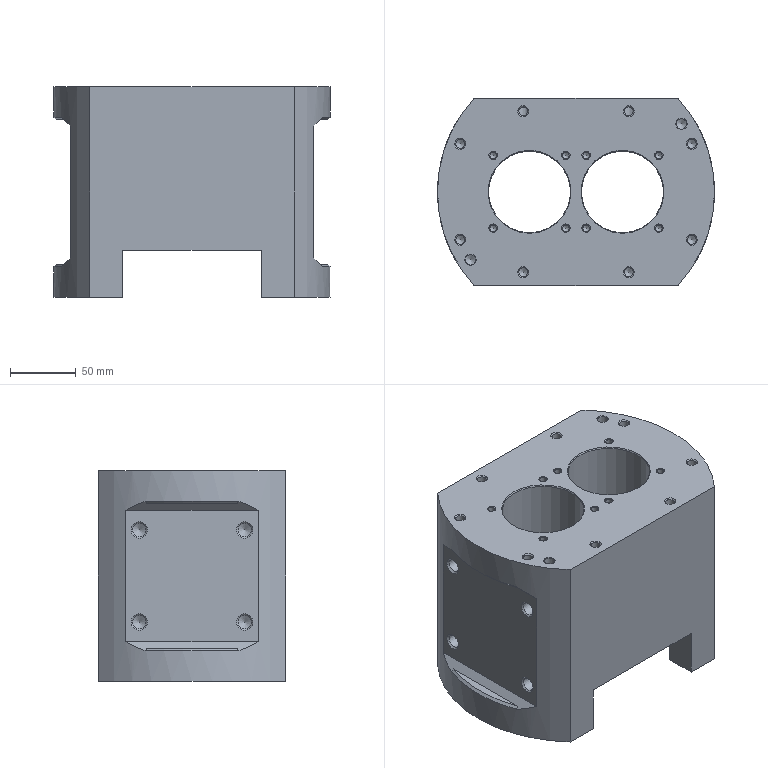NC program | NX | posted with a generic post | part box 210 x 142 x 160 mm
Lines 2091 to 2948 of 4789:
(ZLEVEL_PROFILE , TOOL : D6R0.5)
N4168 T05 M6
N4170 G54
N4172 G17 G0 G90 X-53.624 Y12.863 B0. C0. S6500 M3
N4174 G43 Z30. H5
N4176 Z2.929
N4178 G94 G1 Z-0.071 F1000.
N4180 X-54.42 Y12.281
N4182 G3 X-54.662 Y11.732 R0.6
N4184 G2 X-54.662 Y-11.732 R108.942 F2500.
N4186 G1 X-54.661 Y-11.887 Z-0.088
N4188 Y-12.042 Z-0.106
N4190 X-54.662 Y-12.197 Z-0.124
N4192 X-54.665 Y-12.352 Z-0.141
N4194 G3 X-54.665 Y12.356 R108.252
N4196 G1 X-54.663 Y12.506 Z-0.159
N4198 Y12.657 Z-0.177
N4200 X-54.664 Y12.807 Z-0.194
N4202 X-54.667 Y12.957 Z-0.212
N4204 G2 X-54.667 Y-12.956 R107.872
N4206 G1 X-54.664 Y-13.103 Z-0.23
N4208 X-54.665 Y-13.25 Z-0.247
N4210 Y-13.397 Z-0.265
N4212 X-54.667 Y-13.544 Z-0.283
N4214 G3 X-54.667 Y13.543 R108.056
N4216 G1 X-54.666 Y13.687 Z-0.301
N4218 X-54.667 Y13.832 Z-0.318
N4220 Y13.976 Z-0.336
N4222 X-54.669 Y14.12 Z-0.354
N4224 G2 X-54.668 Y-14.125 R108.36
N4226 G1 X-54.666 Y-14.262 Z-0.371
N4228 Y-14.4 Z-0.389
N4230 X-54.667 Y-14.537 Z-0.407
N4232 X-54.671 Y-14.674 Z-0.424
N4234 G3 X-54.671 Y14.674 R108.329
N4236 G1 X-54.667 Y14.844 Z-0.448
N4238 X-54.668 Y15.014 Z-0.471
N4240 X-54.671 Y15.183 Z-0.495
N4242 G2 X-54.671 Y-15.179 R107.83
N4244 G1 Y-15.344 Z-0.519
N4246 Y-15.508 Z-0.542
N4248 X-54.674 Y-15.672 Z-0.566
N4250 G3 X-54.674 Y15.674 R107.881
N4252 G1 X-54.672 Y15.836 Z-0.589
N4254 Y15.998 Z-0.613
N4256 X-54.675 Y16.159 Z-0.636
N4258 G2 X-54.675 Y-16.159 R107.965
N4260 G1 X-54.673 Y-16.318 Z-0.66
N4262 X-54.674 Y-16.477 Z-0.684
N4264 X-54.675 Y-16.635 Z-0.707
N4266 G3 X-54.675 Y16.633 R108.191
N4268 G1 Y16.79 Z-0.731
N4270 Y16.947 Z-0.754
N4272 X-54.679 Y17.103 Z-0.778
N4274 G2 X-54.678 Y-17.106 R108.255
N4276 G1 X-54.675 Y-17.257 Z-0.801
N4278 X-54.676 Y-17.407 Z-0.825
N4280 X-54.679 Y-17.557 Z-0.849
N4282 G3 X-54.679 Y17.556 R108.476
N4284 G1 X-54.677 Y17.701 Z-0.872
N4286 Y17.846 Z-0.896
N4288 X-54.679 Y17.991 Z-0.919
N4290 G2 X-54.679 Y-17.987 R108.599
N4292 G1 Y-18.125 Z-0.943
N4294 X-54.68 Y-18.263 Z-0.966
N4296 X-54.682 Y-18.401 Z-0.99
N4298 G3 X-54.682 Y18.403 R108.317
N4300 G1 X-54.681 Y18.541 Z-1.014
N4302 Y18.679 Z-1.037
N4304 X-54.685 Y18.816 Z-1.061
N4306 G2 X-54.685 Y-18.815 R108.248
N4308 G1 X-54.682 Y-18.951 Z-1.084
N4310 X-54.683 Y-19.086 Z-1.108
N4312 X-54.686 Y-19.221 Z-1.131
N4314 G3 X-54.686 Y19.221 R108.279
N4316 G1 X-54.684 Y19.354 Z-1.155
N4318 X-54.685 Y19.488 Z-1.179
N4320 X-54.687 Y19.62 Z-1.202
N4322 G2 X-54.687 Y-19.622 R108.38
N4324 G1 X-54.685 Y-19.756 Z-1.226
N4326 Y-19.89 Z-1.249
N4328 X-54.687 Y-20.023 Z-1.273
N4330 G3 X-54.687 Y20.019 R108.652
N4332 G1 X-54.686 Y20.146 Z-1.296
N4334 X-54.687 Y20.274 Z-1.32
N4336 X-54.688 Y20.401 Z-1.344
N4338 G2 X-54.688 Y-20.401 R108.747
N4340 G1 Y-20.526 Z-1.367
N4342 X-54.689 Y-20.651 Z-1.391
N4344 X-54.69 Y-20.775 Z-1.414
N4346 G3 X-54.689 Y20.778 R108.773
N4348 G1 Y20.897 Z-1.438
N4350 X-54.69 Y21.015 Z-1.461
N4352 X-54.691 Y21.134 Z-1.485
N4354 G2 X-54.691 Y-21.132 R108.6
N4356 G1 Y-21.251 Z-1.508
N4358 Y-21.37 Z-1.532
N4360 X-54.693 Y-21.488 Z-1.556
N4362 G3 X-54.693 Y21.49 R108.595
N4364 G1 X-54.692 Y21.608 Z-1.579
N4366 X-54.693 Y21.726 Z-1.603
N4368 X-54.694 Y21.843 Z-1.626
N4370 G2 X-54.694 Y-21.843 R108.602
N4372 G1 Y-22.016 Z-1.662
N4374 X-54.695 Y-22.189 Z-1.697
N4376 G3 X-54.695 Y22.188 R108.586
N4378 G1 Y22.359 Z-1.732
N4380 X-54.696 Y22.53 Z-1.768
N4382 G2 X-52.49 Y-5.881 R108.942
N4384 X-54.696 Y-22.532 R111.727
N4386 G1 X-54.695 Y-22.703 Z-1.803
N4388 X-54.696 Y-22.874 Z-1.838
N4390 G3 X-52.291 Y-2.768 R111.408
N4392 X-54.697 Y22.872 R109.772
N4394 G1 X-54.696 Y23.036 Z-1.874
N4396 X-54.697 Y23.199 Z-1.909
N4398 G2 X-52.184 Y0. R110.754
N4400 X-54.697 Y-23.2 R110.742
N4402 G1 Y-23.361 Z-1.945
N4404 Y-23.523 Z-1.98
N4406 G3 X-52.15 Y-2.768 R111.476
N4408 X-54.697 Y23.525 R110.138
N4410 G1 X-54.696 Y23.683 Z-2.015
N4412 X-54.698 Y23.84 Z-2.051
N4414 G2 X-52.147 Y4.497 R110.747
N4416 X-52.188 Y-5.535 R122.613
N4418 X-54.699 Y-23.836 R112.131
N4420 G1 X-54.698 Y-23.991 Z-2.086
N4422 X-54.7 Y-24.145 Z-2.121
N4424 G3 X-52.12 Y-5.535 R111.408
N4426 X-52.12 Y5.535 R174.408
N4428 X-54.7 Y24.147 R111.521
N4430 G1 X-54.699 Y24.301 Z-2.157
N4432 X-54.702 Y24.454 Z-2.192
N4434 G2 X-52.227 Y8.302 R112.523
N4436 X-52.055 Y4.784 R58.069
N4438 X-52.07 Y-5.535 R256.368
N4440 X-53.483 Y-18.335 R102.106
N4442 X-54.702 Y-24.453 R104.408
N4444 G1 X-54.7 Y-24.608 Z-2.228
N4446 X-54.703 Y-24.761 Z-2.263
N4448 G3 X-52.157 Y-8.302 R112.193
N4450 X-52.023 Y-4.71 R68.447
N4452 X-52.023 Y4.71 R497.71
N4454 X-52.157 Y8.302 R68.447
N4456 X-54.703 Y24.761 R112.204
N4458 G1 X-54.701 Y24.916 Z-2.299
N4460 X-54.704 Y25.069 Z-2.334
N4462 G2 X-52.097 Y8.302 R109.925
N4464 X-52. Y3.907 R99.302
N4466 G1 Y-3.907
N4468 G2 X-52.097 Y-8.302 R99.301
N4470 X-54.704 Y-25.069 R109.989
N4472 G1 X-54.702 Y-25.224 Z-2.37
N4474 X-54.705 Y-25.378 Z-2.405
N4476 G3 X-53.78 Y-21.102 R106.125
N4478 X-52.092 Y-8.994 R103.684
N4480 X-52. Y-5.563 R64.244
N4482 G1 Y4.497
N4484 G3 X-52.056 Y8.302 R101.819
N4486 X-52.268 Y11.07 R47.31
N4488 X-54.705 Y25.376 R113.821
N4490 G1 X-54.703 Y25.529 Z-2.441
N4492 X-54.706 Y25.681 Z-2.476
N4494 G2 X-52.203 Y11.125 R114.465
N4496 X-52.021 Y8.052 R33.208
N4498 G1 X-52.002 Y6.573
N4500 X-52.001 Y6.227
N4502 X-52. Y6.031
N4504 Y-6.04
N4506 X-52.002 Y-6.573
N4508 X-52.021 Y-8.036
N4510 G2 X-52.207 Y-11.158 R33.543
N4512 X-54.705 Y-25.683 R115.071
N4514 G1 X-54.704 Y-25.831 Z-2.512
N4516 X-54.706 Y-25.978 Z-2.547
N4518 G3 X-52.164 Y-11.416 R115.432
N4520 X-52.002 Y-7.611 R42.565
N4522 G1 X-52.001 Y-7.265
N4524 X-52. Y-7.142
N4526 Y7.145
N4528 X-52.001 Y7.265
N4530 X-52.002 Y7.611
N4532 G3 X-52.164 Y11.416 R42.565
N4534 X-54.706 Y25.977 R114.96
N4536 G1 Y26.124 Z-2.583
N4538 X-54.707 Y26.27 Z-2.619
N4540 G2 X-52.137 Y11.762 R113.314
N4542 X-52.003 Y8.648 R35.799
N4544 G1 X-52.001 Y8.302
N4546 X-52. Y8.103
N4548 Y-8.105
N4550 X-52.001 Y-8.302
N4552 X-52.003 Y-8.648
N4554 G2 X-52.281 Y-13.113 R35.799
N4556 X-54.707 Y-26.269 R115.866
N4558 G1 Y-26.414 Z-2.654
N4560 X-54.709 Y-26.558 Z-2.69
N4562 G3 X-52.181 Y-12.751 R112.204
N4564 X-52.021 Y-10.354 R23.254
N4566 G1 X-52. Y-8.965
N4568 Y8.961
N4570 X-52.017 Y10.229
N4572 G3 X-52.185 Y12.78 R24.281
N4574 G1 X-52.311 Y13.837
N4576 G3 X-54.709 Y26.561 R116.193
N4578 G1 X-54.708 Y26.701 Z-2.725
N4580 X-54.711 Y26.841 Z-2.761
N4582 G2 X-52.271 Y14.084 R116.39
N4584 X-52. Y10.016 R30.646
N4586 G1 Y-10.011
N4588 G2 X-52.272 Y-14.089 R30.724
N4590 X-54.711 Y-26.838 R116.147
N4592 G1 X-54.71 Y-26.978 Z-2.797
N4594 X-54.712 Y-27.116 Z-2.832
N4596 G3 X-52.169 Y-13.837 R115.357
N4598 X-52. Y-10.472 R29.781
N4600 G1 Y10.469
N4602 G3 X-52.169 Y13.837 R29.789
N4604 X-54.712 Y27.117 R115.492
N4606 G1 X-54.711 Y27.256 Z-2.868
N4608 X-54.713 Y27.394 Z-2.904
N4610 G2 X-52.146 Y14.183 R115.213
N4612 X-52. Y11.149 R28.716
N4614 G1 Y-11.146
N4616 G2 X-52.146 Y-14.183 R28.725
N4618 X-54.713 Y-27.394 R115.148
N4620 G1 X-54.712 Y-27.533 Z-2.939
N4622 X-54.713 Y-27.671 Z-2.975
N4624 G3 X-52.174 Y-14.875 R114.201
N4626 X-52.023 Y-13.032 R16.656
N4628 G1 X-52.002 Y-12.108
N4630 X-52. Y-11.762
N4632 Y11.762
N4634 X-52.002 Y12.108
N4636 X-52.023 Y13.032
N4638 G3 X-52.174 Y14.875 R16.656
N4640 X-54.713 Y27.671 R114.156
N4642 G1 X-54.714 Y27.809 Z-3.011
N4644 X-54.716 Y27.948 Z-3.047
N4646 G2 X-52.354 Y16.605 R116.379
N4648 G1 X-52.209 Y15.604
N4650 G2 X-52. Y12.71 R20.134
N4652 G1 Y-12.711
N4654 G2 X-52.209 Y-15.603 R20.128
N4656 X-54.716 Y-27.949 R112.331
N4658 G1 X-54.715 Y-28.088 Z-3.082
N4660 X-54.717 Y-28.226 Z-3.118
N4662 G3 X-52.284 Y-16.605 R117.119
N4664 X-52. Y-12.971 R21.432
N4666 G1 Y12.966
N4668 G3 X-52.284 Y16.605 R21.439
N4670 X-54.718 Y28.225 R116.832
N4672 G1 X-54.716 Y28.362 Z-3.154
N4674 X-54.719 Y28.498 Z-3.19
N4676 G2 X-52.266 Y16.951 R118.71
N4678 X-52. Y13.522 R20.174
N4680 G1 Y-13.519
N4682 G2 X-52.266 Y-16.951 R20.179
N4684 X-54.718 Y-28.499 R119.042
N4686 G1 X-54.717 Y-28.633 Z-3.225
N4688 X-54.719 Y-28.766 Z-3.261
N4690 G3 X-52.145 Y-16.605 R117.466
N4692 X-52. Y-14.05 R21.711
N4694 G1 Y14.051
N4696 G3 X-52.145 Y16.605 R21.711
N4698 X-54.719 Y28.765 R117.28
N4700 G1 Y28.898 Z-3.297
N4702 X-54.72 Y29.03 Z-3.333
N4704 G2 X-52.185 Y17.297 R117.957
N4706 X-52.003 Y14.875 R16.386
N4708 G1 X-52. Y14.529
N4710 Y-14.529
N4712 X-52.003 Y-14.875
N4714 G2 X-52.223 Y-17.539 R16.386
N4716 X-54.72 Y-29.03 R117.614
N4718 G1 X-54.721 Y-29.162 Z-3.369
N4720 X-54.723 Y-29.293 Z-3.405
N4722 G3 X-52.253 Y-18.146 R118.37
N4724 X-52. Y-15.055 R17.598
N4726 G1 Y15.06
N4728 G3 X-52.174 Y17.643 R17.583
N4730 X-54.723 Y29.295 R116.908
N4732 G1 X-54.721 Y29.424 Z-3.441
N4734 X-54.724 Y29.553 Z-3.476
N4736 G2 X-52.205 Y18.233 R116.076
N4738 X-52. Y15.812 R14.397
N4740 G1 Y-15.812
N4742 G2 X-52.205 Y-18.233 R14.405
N4744 X-54.724 Y-29.551 R115.725
N4746 G1 X-54.723 Y-29.678 Z-3.512
N4748 X-54.725 Y-29.804 Z-3.548
N4750 G3 X-52.266 Y-19.022 R119.178
N4752 X-52. Y-16.044 R16.838
N4754 G1 Y16.038
N4756 G3 X-52.268 Y19.035 R16.902
N4758 X-54.725 Y29.806 R120.043
N4760 G1 Y29.931 Z-3.584
N4762 X-54.726 Y30.057 Z-3.62
N4764 G2 X-52.259 Y19.372 R119.21
N4766 X-52. Y16.451 R15.402
N4768 G1 Y-16.45
N4770 G2 X-52.259 Y-19.372 R15.404
N4772 X-54.726 Y-30.056 R119.032
N4774 G1 Y-30.182 Z-3.656
N4776 X-54.728 Y-30.308 Z-3.692
N4778 G3 X-52.268 Y-19.834 R120.353
N4780 X-52. Y-16.892 R15.521
N4782 G1 Y16.889
N4784 G3 X-52.188 Y19.372 R15.529
N4786 X-54.728 Y30.308 R118.6
N4788 G1 Y30.434 Z-3.728
N4790 X-54.73 Y30.559 Z-3.764
N4792 G2 X-52.18 Y19.718 R119.547
N4794 X-52. Y17.297 R15.111
N4796 G1 Y-17.297
N4798 G2 X-52.274 Y-20.254 R15.111
N4800 X-54.73 Y-30.56 R122.48
N4802 G1 X-54.729 Y-30.686 Z-3.8
N4804 X-54.73 Y-30.812 Z-3.836
N4806 G3 X-52.25 Y-20.469 R120.933
N4808 X-52. Y-17.737 R13.747
N4810 G1 Y17.734
N4812 G3 X-52.178 Y20.064 R13.754
N4814 X-54.73 Y30.811 R118.632
N4816 G1 X-54.731 Y30.937 Z-3.872
N4818 X-54.733 Y31.063 Z-3.908
N4820 G2 X-52.176 Y20.41 R117.84
N4822 X-52. Y18.145 R13.425
N4824 G1 Y-18.142
N4826 G2 X-52.252 Y-20.83 R13.431
N4828 X-54.732 Y-31.064 R120.523
N4830 G1 X-54.731 Y-31.188 Z-3.944
N4832 X-54.734 Y-31.311 Z-3.98
N4834 G3 X-52.252 Y-21.18 R120.416
N4836 X-52. Y-18.544 R13.025
N4838 G1 Y18.541
N4840 G3 X-52.174 Y20.756 R13.029
N4842 X-54.734 Y31.31 R117.68
N4844 G1 Y31.432 Z-4.016
N4846 X-54.735 Y31.553 Z-4.052
N4848 G2 X-52.239 Y21.448 R119.025
N4850 X-52. Y18.934 R12.234
N4852 G1 Y-18.932
N4854 G2 X-52.239 Y-21.448 R12.237
N4856 X-54.735 Y-31.554 R119.24
N4858 G1 Y-31.675 Z-4.088
N4860 X-54.737 Y-31.795 Z-4.124
N4862 G3 X-52.268 Y-21.961 R123.325
N4864 X-52. Y-19.352 R12.828
N4866 G1 Y19.352
N4868 G3 X-52.268 Y21.961 R12.828
N4870 X-54.737 Y31.795 R123.29
N4872 G1 Y31.916 Z-4.16
N4874 X-54.739 Y32.036 Z-4.196
N4876 G2 X-52.271 Y22.32 R124.24
N4878 X-52. Y19.73 R12.517
N4880 G1 Y-19.73
N4882 G2 X-52.271 Y-22.32 R12.522
N4884 X-54.739 Y-32.036 R124.057
N4886 G1 X-54.738 Y-32.155 Z-4.233
N4888 X-54.74 Y-32.274 Z-4.269
N4890 G3 X-52.236 Y-22.486 R124.486
N4892 X-52. Y-20.061 R11.823
N4894 G1 Y20.059
N4896 G3 X-52.236 Y22.486 R11.826
N4898 X-54.74 Y32.275 R124.82
N4900 G1 X-54.739 Y32.393 Z-4.305
N4902 X-54.741 Y32.511 Z-4.341
N4904 G2 X-52.172 Y22.486 R121.159
N4906 X-52. Y20.41 R11.611
N4908 G1 Y-20.41
N4910 G2 X-52.265 Y-22.965 R11.611
N4912 X-54.741 Y-32.509 R124.985
N4914 G1 X-54.742 Y-32.626 Z-4.377
N4916 X-54.744 Y-32.741 Z-4.413
N4918 G3 X-52.25 Y-23.178 R119.385
N4920 X-52. Y-20.756 R10.655
N4922 G1 Y20.756
N4924 G3 X-52.25 Y23.178 R10.655
N4926 X-54.744 Y32.742 R119.49
N4928 G1 Y32.858 Z-4.45
N4930 X-54.745 Y32.973 Z-4.486
N4932 G2 X-52.257 Y23.524 R118.651
N4934 X-52. Y21.102 R10.304
N4936 G1 Y-21.102
N4938 G2 X-52.257 Y-23.524 R10.304
N4940 X-54.745 Y-32.973 R118.658
N4942 G1 Y-33.089 Z-4.522
N4944 X-54.746 Y-33.205 Z-4.558
N4946 G3 X-52.263 Y-23.87 R119.333
N4948 X-52. Y-21.471 R10.23
N4950 G1 Y21.469
N4952 G3 X-52.263 Y23.87 R10.231
N4954 X-54.747 Y33.205 R118.547
N4956 G1 Y33.321 Z-4.595
N4958 X-54.749 Y33.436 Z-4.631
N4960 G2 X-52.27 Y24.216 R119.941
N4962 X-52. Y21.808 R10.252
N4964 G1 Y-21.808
N4966 G2 X-52.27 Y-24.216 R10.252
N4968 X-54.749 Y-33.437 R120.301
N4970 G1 Y-33.554 Z-4.667
N4972 X-54.75 Y-33.67 Z-4.703
N4974 G3 X-52.281 Y-24.598 R126.62
N4976 X-52. Y-22.146 R10.821
N4978 G1 Y22.145
N4980 G3 X-52.281 Y24.594 R10.821
N4982 X-54.751 Y33.668 R125.32
N4984 G1 Y33.784 Z-4.74
N4986 X-54.752 Y33.899 Z-4.776
N4988 G2 X-52.283 Y24.907 R127.611
N4990 X-52. Y22.469 R10.339
N4992 G1 Y-22.471
N4994 G2 X-52.283 Y-24.907 R10.34
N4996 X-54.751 Y-33.902 R128.786
N4998 G1 X-54.752 Y-34.017 Z-4.812
N5000 X-54.753 Y-34.131 Z-4.849
N5002 G3 X-52.286 Y-25.238 R131.317
N5004 X-52. Y-22.792 R10.385
N5006 G1 Y22.795
N5008 G3 X-52.213 Y24.907 R10.384
N5010 X-54.754 Y34.127 R127.364
N5012 G1 Y34.241 Z-4.885
N5014 X-54.756 Y34.354 Z-4.921
N5016 G2 X-52.224 Y25.253 R129.062
N5018 X-52. Y23.111 R9.869
N5020 G1 Y-23.113
N5022 G2 X-52.278 Y-25.489 R9.867
N5024 X-54.754 Y-34.359 R134.317
N5026 G1 Y-34.473 Z-4.958
N5028 X-54.755 Y-34.586 Z-4.994
N5030 G3 X-52.276 Y-25.771 R134.833
N5032 X-52. Y-23.426 R9.607
N5034 G1 Y23.427
N5036 G3 X-52.164 Y25.253 R9.605
N5038 X-54.757 Y34.58 R122.15
N5040 G1 X-54.758 Y34.693 Z-5.03
N5042 X-54.759 Y34.806 Z-5.067
N5044 G2 X-52.255 Y25.945 R127.468
N5046 X-52. Y23.736 R9.005
N5048 G1 Y-23.736
N5050 G2 X-52.255 Y-25.945 R9.005
N5052 X-54.757 Y-34.815 R131.929
N5054 G1 X-54.751 Y-34.913 Z-5.103
N5056 X-54.746 Y-35.011 Z-5.14
N5058 G3 X-52.271 Y-26.291 R136.064
N5060 X-52. Y-24.044 R8.714
N5062 G1 Y24.042
N5064 G3 X-52.271 Y26.291 R8.728
N5066 X-54.75 Y35.005 R130.083
N5068 G1 X-54.726 Y35.165 Z-5.213
N5070 G2 X-52.287 Y26.637 R137.601
N5072 X-52. Y24.347 R8.741
N5074 G1 Y-24.43
N5076 G2 X-52.25 Y-26.486 R8.593
N5078 X-54.092 Y-33.115 R116.776
N5080 G1 X-54.657 Y-34.94
N5082 X-54.723 Y-35.17
N5084 X-54.691 Y-35.317 Z-5.285
N5086 G2 X-54.318 Y-34.068 R37.514
N5088 G3 X-52.26 Y-26.811 R121.891
N5090 X-52. Y-24.703 R8.674
N5092 G1 Y24.7
N5094 G3 X-52.26 Y26.81 R8.702
N5096 X-53.945 Y32.864 R118.382
N5098 G1 X-54.05 Y33.21
N5100 X-54.591 Y34.94
N5102 X-54.694 Y35.314
N5104 X-54.647 Y35.431 Z-5.358
N5106 X-54.615 Y35.286
N5108 X-54.305 Y34.248
N5110 X-54.196 Y33.902
N5112 G2 X-52.267 Y27.12 R124.237
N5114 X-52. Y24.985 R8.674
N5116 G1 Y-24.994
N5118 G2 X-52.265 Y-27.113 R8.596
N5120 X-54.415 Y-34.594 R126.303
N5122 G1 X-54.613 Y-35.286
N5124 X-54.646 Y-35.432
N5126 X-54.587 Y-35.551 Z-5.431
N5128 G2 X-54.417 Y-34.817 R4.459
N5130 G3 X-52.289 Y-27.505 R135.792
N5132 X-52. Y-25.249 R8.941
N5134 G1 Y25.249
N5136 G3 X-52.292 Y27.516 R8.943
N5138 X-54.465 Y34.981 R144.574
N5140 G2 X-54.586 Y35.551 R2.928
N5142 G1 X-54.517 Y35.674 Z-5.504
N5144 G3 X-54.382 Y34.94 R2.785
N5146 G2 X-52.291 Y27.78 R148.685
N5148 X-52. Y25.55 R8.704
N5150 G1 Y-25.549
N5152 G2 X-52.289 Y-27.774 R8.708
N5154 X-54.385 Y-34.94 R142.859
N5156 G3 X-54.519 Y-35.673 R3.003
N5158 G1 X-54.451 Y-35.8 Z-5.576
N5160 G2 X-54.318 Y-34.94 R3.035
N5162 G3 X-52.274 Y-27.972 R138.856
N5164 X-52. Y-25.868 R8.209
N5166 G1 Y25.865
N5168 G3 X-52.275 Y27.974 R8.237
N5170 X-53.989 Y33.902 R136.846
N5172 G1 X-54.208 Y34.594
N5174 X-54.314 Y34.94
N5176 G2 X-54.448 Y35.803 R2.806
N5178 G1 X-54.376 Y35.924 Z-5.647
N5180 X-54.341 Y35.286
N5182 X-54.246 Y34.94
N5184 X-53.64 Y32.984
N5186 G2 X-52.272 Y28.224 R120.035
N5188 X-52. Y26.142 R8.123
N5190 G1 Y-26.144
N5192 G2 X-52.274 Y-28.231 R8.092
N5194 X-54.225 Y-34.855 R134.623
N5196 G3 X-54.379 Y-35.921 R3.213
N5198 G1 X-54.313 Y-36.048 Z-5.719
N5200 X-54.273 Y-35.286
N5202 G2 X-54.045 Y-34.504 R15.284
N5204 G3 X-52.244 Y-28.367 R128.46
N5206 X-52. Y-26.345 R7.905
N5208 G1 Y26.437
N5210 G3 X-52.282 Y28.505 R7.716
N5212 G1 X-53.014 Y31.134
N5214 X-53.117 Y31.48
N5216 X-54.178 Y34.94
N5218 X-54.275 Y35.286
N5220 X-54.315 Y36.15
N5222 X-54.274 Z-5.754
N5224 X-54.241 Z-5.79
N5226 X-54.21 Y35.286
N5228 X-52.946 Y31.134
N5230 X-52.844 Y30.788
N5232 X-52.271 Y28.713
N5234 X-52.183 Y28.367
N5236 G2 X-52. Y26.613 R7.916
N5238 G1 Y-26.611
N5240 G2 X-52.271 Y-28.713 R7.72
N5242 X-54.043 Y-34.709 R125.296
N5244 G3 X-54.206 Y-35.286 R8.237
N5246 G1 X-54.247 Y-36.183
N5248 X-54.178 Y-36.318 Z-5.861
N5250 X-54.14 Y-35.286
N5252 G2 X-53.976 Y-34.71 R8.337
N5254 G3 X-52.263 Y-28.931 R122.225
N5256 X-52. Y-26.947 R7.614
N5258 G1 Y26.959
N5260 G3 X-52.269 Y28.948 R7.486
N5262 G1 X-52.776 Y30.788
N5264 X-52.879 Y31.134
N5266 X-54.145 Y35.286
N5268 X-54.173 Y36.329
N5270 X-54.139 Y36.421 Z-5.896
N5272 X-54.105 Y36.513 Z-5.932
N5274 X-54.104 Y36.323
N5276 X-54.081 Y35.459
N5278 Y35.286
N5280 G2 X-52.277 Y29.23 R168.559
N5282 X-52. Y27.194 R7.614
N5284 G1 Y-27.19
N5286 G2 X-52.269 Y-29.204 R7.668
N5288 X-53.923 Y-34.751 R121.212
N5290 G3 X-54.073 Y-35.286 R7.18
N5292 G1 X-54.108 Y-36.323
N5294 X-54.111 Y-36.507
N5296 X-54.073 Y-36.603 Z-5.967
N5298 X-54.04 Y-36.698 Z-6.002
N5300 X-54.007 Y-35.286
N5302 G2 X-53.857 Y-34.753 R7.33
N5304 G3 X-52.257 Y-29.405 R120.834
N5306 X-52. Y-27.394 R7.624
N5308 G1 Y27.396
N5310 G3 X-52.257 Y29.405 R7.623
N5312 X-54.021 Y35.286 R142.445
N5314 G1 X-54.037 Y36.702
N5316 X-54.001 Y36.797 Z-6.038
N5318 X-53.97 Y36.892 Z-6.073
N5320 X-53.961 Y35.286
N5322 G2 X-52.29 Y29.78 R138.956
N5324 X-52. Y27.68 R7.761
N5326 G1 Y-27.65
N5328 G2 X-52.284 Y-29.751 R7.539
N5330 X-53.897 Y-35.086 R125.171
N5332 G3 X-53.943 Y-35.356 R0.927
N5334 G1 X-53.972 Y-36.889
N5336 X-53.933 Y-36.985 Z-6.108
N5338 X-53.901 Y-37.08 Z-6.144
N5340 X-53.879 Y-35.286
N5342 X-53.783 Y-34.94
N5344 G3 X-52.311 Y-30.097 R134.043
N5346 X-52. Y-27.905 R7.722
N5348 G1 Y27.904
N5350 G3 X-52.311 Y30.097 R7.723
N5352 X-53.896 Y35.286 R134.797
N5354 G1 X-53.899 Y37.081
N5356 X-53.863 Y37.175 Z-6.179
N5358 X-53.83 Y37.269 Z-6.214
N5360 X-53.822 Y35.632
N5362 X-53.828 Y35.286
N5364 G2 X-52.338 Y30.442 R153.767
N5366 X-52. Y28.155 R7.84
N5368 G1 Y-28.153
N5370 G2 X-52.338 Y-30.442 R7.84
N5372 X-53.817 Y-35.286 R258.336
N5374 G1 X-53.831 Y-37.268
N5376 X-53.793 Y-37.361 Z-6.25
N5378 X-53.76 Y-37.455 Z-6.285
N5380 X-53.748 Y-35.459
N5382 X-53.758 Y-35.27
N5384 G3 X-52.293 Y-30.518 R143.435
N5386 X-52. Y-28.448 R7.451
N5388 G1 Y28.448
N5390 G3 X-52.294 Y30.519 R7.452
N5392 X-53.758 Y35.271 R144.455
N5394 G1 Y35.375
N5396 X-53.756 Y35.632
N5398 X-53.757 Y37.361
N5400 X-53.76 Y37.455
N5402 X-53.722 Y37.548 Z-6.321
N5404 X-53.688 Y37.64 Z-6.356
N5406 X-53.687 Y35.572
N5408 Y35.266
N5410 G2 X-52.289 Y30.732 R151.472
N5412 X-52. Y28.705 R7.249
N5414 G1 Y-28.705
N5416 G2 X-52.289 Y-30.731 R7.249
N5418 X-53.687 Y-35.266 R151.472
N5420 G1 Y-35.537
N5422 X-53.682 Y-35.58
N5424 X-53.688 Y-37.64
N5426 X-53.651 Y-37.733 Z-6.391
N5428 X-53.621 Y-37.825 Z-6.427
N5430 X-53.616 Y-35.768
N5432 Y-35.254
N5434 G3 X-52.285 Y-30.951 R153.179
N5436 X-52. Y-28.963 R7.065
N5438 G1 Y28.957
N5440 G3 X-52.287 Y30.957 R7.107
N5442 X-53.616 Y35.254 R153.179
N5444 G1 Y35.768
N5446 Y37.707
N5448 X-53.621 Y37.825
N5450 X-53.581 Y37.918 Z-6.462
N5452 X-53.548 Y38.011 Z-6.497
N5454 X-53.545 Y37.707
N5456 X-53.546 Y35.963
N5458 Y35.242
N5460 G2 X-52.274 Y31.134 R136.959
N5462 X-52. Y29.132 R6.872
N5464 G1 Y-29.131
N5466 G2 X-52.274 Y-31.134 R6.873
N5468 X-53.546 Y-35.242 R136.959
N5470 G1 X-53.545 Y-35.977
N5472 X-53.548 Y-38.01
N5474 X-53.51 Y-38.103 Z-6.533
N5476 X-53.479 Y-38.196 Z-6.568
N5478 X-53.475 Y-38.053
N5480 X-53.473 Y-36.323
N5482 X-53.475 Y-36.156
N5484 Y-35.23
N5486 G3 X-52.272 Y-31.349 R122.716
N5488 X-52. Y-29.442 R6.807
N5490 G1 Y29.442
N5492 G3 X-52.272 Y31.349 R6.807
N5494 X-53.475 Y35.23 R122.716
N5496 G1 Y36.156
N5498 X-53.474 Y36.323
N5500 X-53.475 Y38.053
N5502 X-53.479 Y38.196
N5504 X-53.439 Y38.289 Z-6.603
N5506 X-53.405 Y38.381 Z-6.639
N5508 X-53.404 Y36.348
N5510 Y35.218
N5512 G2 X-52.282 Y31.611 R123.63
N5514 X-52. Y29.655 R6.923
N5516 G1 Y-29.655
N5518 G2 X-52.282 Y-31.611 R6.923
N5520 X-53.404 Y-35.218 R123.63
N5522 G1 Y-36.348
N5524 X-53.405 Y-38.381
N5526 X-53.369 Y-38.472 Z-6.674
N5528 X-53.337 Y-38.563 Z-6.709
N5530 X-53.333 Y-38.399
N5532 Y-36.538
N5534 Y-35.206
N5536 G3 X-52.28 Y-31.826 R116.891
N5538 X-52. Y-29.843 R6.757
N5540 G1 Y29.843
N5542 G3 X-52.28 Y31.826 R6.756
N5544 X-53.333 Y35.206 R116.891
N5546 G1 Y36.539
N5548 Y38.399
N5550 X-53.337 Y38.563
N5552 X-53.298 Y38.653 Z-6.745
N5554 X-53.263 Y38.744 Z-6.78
N5556 Y36.73
N5558 Y35.194
N5560 G2 X-52.279 Y32.042 R103.544
N5562 X-52. Y30.112 R6.826
N5564 G1 Y-30.112
N5566 G2 X-52.279 Y-32.042 R6.826
N5568 X-53.263 Y-35.194 R103.544
N5570 G1 Y-36.73
N5572 Y-38.744
N5574 X-53.227 Y-38.833 Z-6.816
N5576 X-53.196 Y-38.922 Z-6.851
N5578 X-53.192 Y-38.745
N5580 X-53.191 Y-37.015
N5582 X-53.192 Y-36.669
N5584 Y-35.181
N5586 G3 X-52.286 Y-32.297 R103.247
N5588 X-52. Y-30.334 R6.875
N5590 G1 Y30.334
N5592 G3 X-52.288 Y32.301 R6.868
N5594 X-53.192 Y35.181 R109.668
N5596 G1 Y36.669
N5598 X-53.191 Y36.921
N5600 X-53.192 Y38.745
N5602 X-53.196 Y38.922
N5604 X-53.157 Y39.011 Z-6.886
N5606 X-53.122 Y39.1 Z-6.922
N5608 X-53.12 Y37.108
N5610 X-53.121 Y37.015
N5612 Y35.169
N5614 X-52.389 Y32.864
N5616 X-52.286 Y32.518
N5618 G2 X-52. Y30.536 R6.74
N5620 G1 Y-30.536
N5622 G2 X-52.286 Y-32.518 R6.74
N5624 G1 X-52.389 Y-32.864
N5626 X-53.121 Y-35.169
N5628 Y-37.015
N5630 X-53.12 Y-37.108
N5632 X-53.122 Y-39.1
N5634 X-53.086 Y-39.189 Z-6.957
N5636 X-53.052 Y-39.278 Z-6.992
N5638 X-53.051 Y-39.091
N5640 X-53.049 Y-37.361
N5642 X-53.051 Y-37.015
N5644 X-53.05 Y-35.147
N5646 X-52.426 Y-33.21
N5648 X-52.322 Y-32.864
N5650 G3 X-52. Y-30.763 R6.875
N5652 G1 Y30.764
N5654 G3 X-52.322 Y32.864 R6.874
N5656 G1 X-52.426 Y33.21
N5658 X-53.05 Y35.147
N5660 X-53.051 Y37.015
N5662 X-53.049 Y37.361
N5664 X-53.051 Y39.091
N5666 X-53.052 Y39.278
N5668 X-53.015 Y39.367 Z-7.028
N5670 X-52.981 Y39.456 Z-7.063
N5672 X-52.978 Y37.479
N5674 X-52.98 Y37.361
N5676 Y35.144
N5678 X-52.359 Y33.21
N5680 G2 X-52. Y30.991 R6.989
N5682 G1 Y-30.989
N5684 G2 X-52.359 Y-33.21 R6.989
N5686 G1 X-52.98 Y-35.144
N5688 Y-37.361
N5690 X-52.981 Y-39.456
N5692 X-52.945 Y-39.545 Z-7.098
N5694 X-52.914 Y-39.634 Z-7.134
N5696 X-52.909 Y-39.437
N5698 Y-37.361
N5700 Y-35.121
N5702 X-52.292 Y-33.21
N5704 X-52.256 Y-33.084
N5706 G3 X-52. Y-31.252 R6.687
N5708 G1 Y31.252
N5710 G3 X-52.256 Y33.084 R6.687
N5712 G1 X-52.292 Y33.21
N5714 X-52.909 Y35.121
N5716 Y37.361
N5718 Y39.437
N5720 X-52.914 Y39.634
N5722 X-52.874 Y39.723 Z-7.169
N5724 X-52.84 Y39.811 Z-7.204
N5726 X-52.838 Y39.783
N5728 X-52.837 Y37.848
N5730 X-52.838 Y37.707
N5732 Y35.109
N5734 X-52.337 Y33.556
N5736 X-52.303 Y33.448
N5738 G2 X-52. Y31.482 R6.541
N5740 G1 Y-31.482
N5742 G2 X-52.303 Y-33.448 R6.54
N5744 G1 X-52.337 Y-33.556
N5746 X-52.838 Y-35.109
N5748 Y-37.707
N5750 X-52.837 Y-37.848
N5752 X-52.838 Y-39.783
N5754 X-52.84 Y-39.811
N5756 X-52.803 Y-39.898 Z-7.24
N5758 X-52.772 Y-39.985 Z-7.275
N5760 X-52.768 Y-39.783
N5762 Y-38.028
N5764 X-52.767 Y-35.096
N5766 X-52.27 Y-33.556
N5768 X-52.227 Y-33.402
N5770 G3 X-52. Y-31.719 R6.341
N5772 G1 Y31.719
N5774 G3 X-52.227 Y33.402 R6.341
N5776 G1 X-52.27 Y33.556
N5778 X-52.767 Y35.096
N5780 X-52.768 Y38.029
N5782 Y39.783
N5784 X-52.772 Y39.985
N5786 X-52.732 Y40.072 Z-7.31
N5788 X-52.698 Y40.158 Z-7.346
N5790 X-52.697 Y38.21
N5792 Y35.094
N5794 X-52.209 Y33.556
N5796 G2 X-52. Y31.874 R6.528
N5798 G1 Y-31.874
N5800 G2 X-52.209 Y-33.556 R6.528
N5802 G1 X-52.697 Y-35.094
N5804 Y-38.21
N5806 X-52.698 Y-40.158
N5808 X-52.662 Y-40.244 Z-7.381
N5810 X-52.63 Y-40.329 Z-7.417
N5812 X-52.626 Y-40.129
N5814 X-52.625 Y-38.399
N5816 X-52.626 Y-38.053
N5818 Y-35.071
N5820 X-52.305 Y-34.076
N5822 G3 X-52. Y-32.142 R6.297
N5824 G1 Y32.142
N5826 G3 X-52.305 Y34.076 R6.298
N5828 G1 X-52.626 Y35.071
N5830 Y38.053
N5832 X-52.625 Y38.399
N5834 X-52.626 Y40.129
N5836 X-52.63 Y40.329
N5838 X-52.591 Y40.415 Z-7.452
N5840 X-52.557 Y40.5 Z-7.487
N5842 X-52.554 Y38.572
N5844 X-52.556 Y38.399
N5846 Y35.069
N5848 X-52.266 Y34.143
N5850 G2 X-52. Y32.399 R5.848
N5852 G1 Y-32.399
N5854 G2 X-52.266 Y-34.143 R5.848
N5856 G1 X-52.556 Y-35.069
N5858 Y-38.399
N5860 X-52.554 Y-38.572
N5862 X-52.557 Y-40.5
N5864 X-52.52 Y-40.586 Z-7.523
N5866 X-52.488 Y-40.671 Z-7.558
N5868 X-52.485 Y-40.475
N5870 X-52.484 Y-38.745
N5872 X-52.485 Y-38.399
N5874 X-52.484 Y-35.046
N5876 X-52.297 Y-34.46